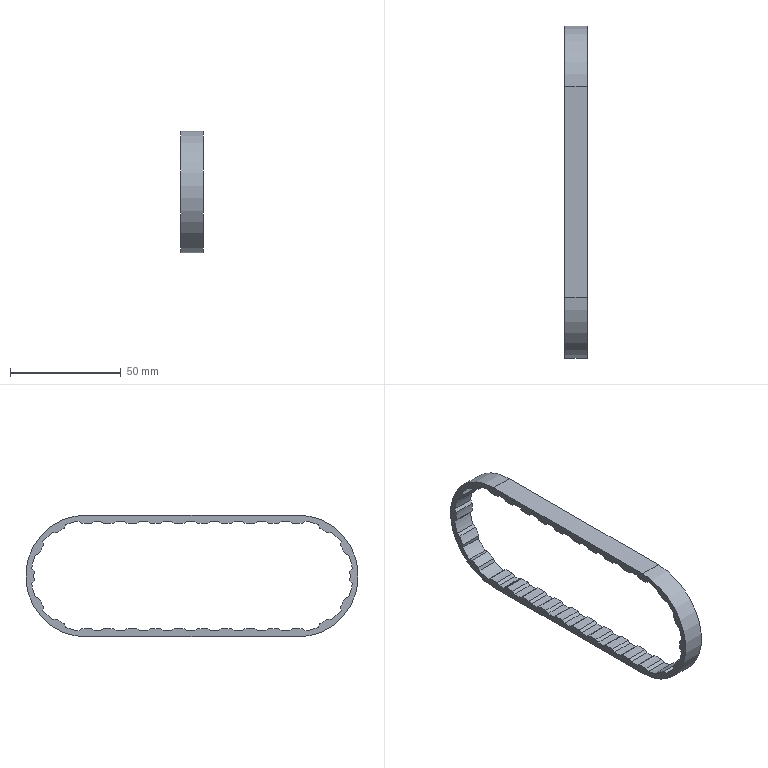Part | NX | features CPROJ 6, DATUM_CSYS 4, EXTRUDE 3, SKETCH 3, EXTRACT_BODY 2, TRIM BODY 2, Container 1, Delete Body 1, Geometry Instance 1, Pattern Geometry 1, UNITE 1 | 1 solid | 128 faces | box 10 x 150 x 55 mm | volume 11245 mm3 | plane 98 | cylinder 30 | commonest cylinder face diameters 47.525 x14 50 x14 55 x2